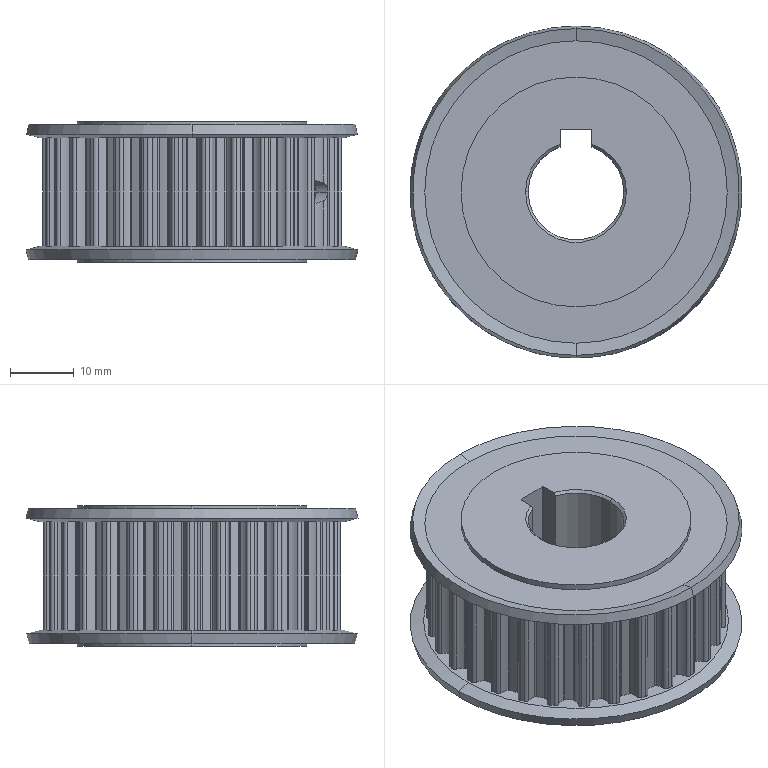Part | SolidWorks | features BaseBody 1 | 1 solid | 338 faces | box 52 x 52 x 22 mm | volume 31133 mm3 | cylinder 293 | plane 27 | cone 18 | commonest cylinder face diameters 1.1 x73 0.5 x72 6.55 x68 43.25 x32 46.79 x31 4.134 x8